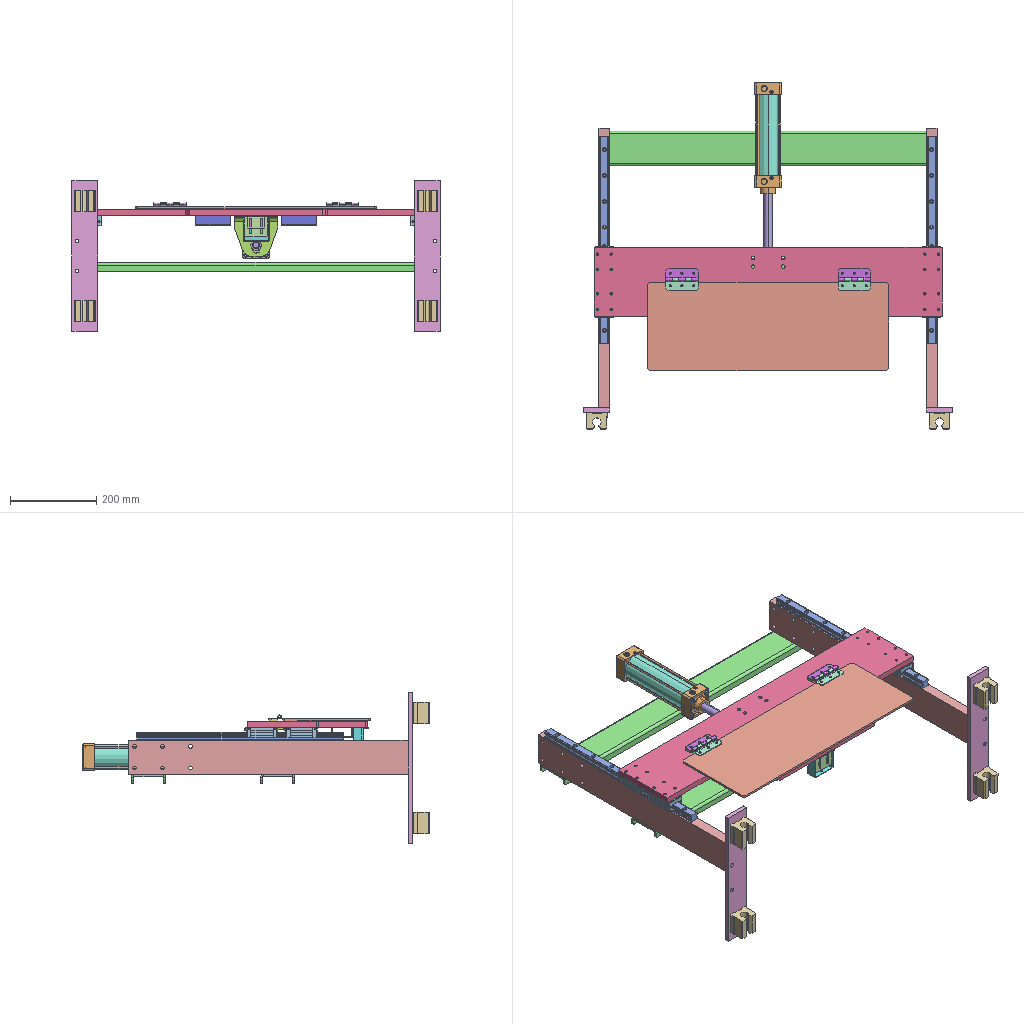Assembly | SolidWorks | 24 different items | 39 placed | box 855 x 804 x 350 mm
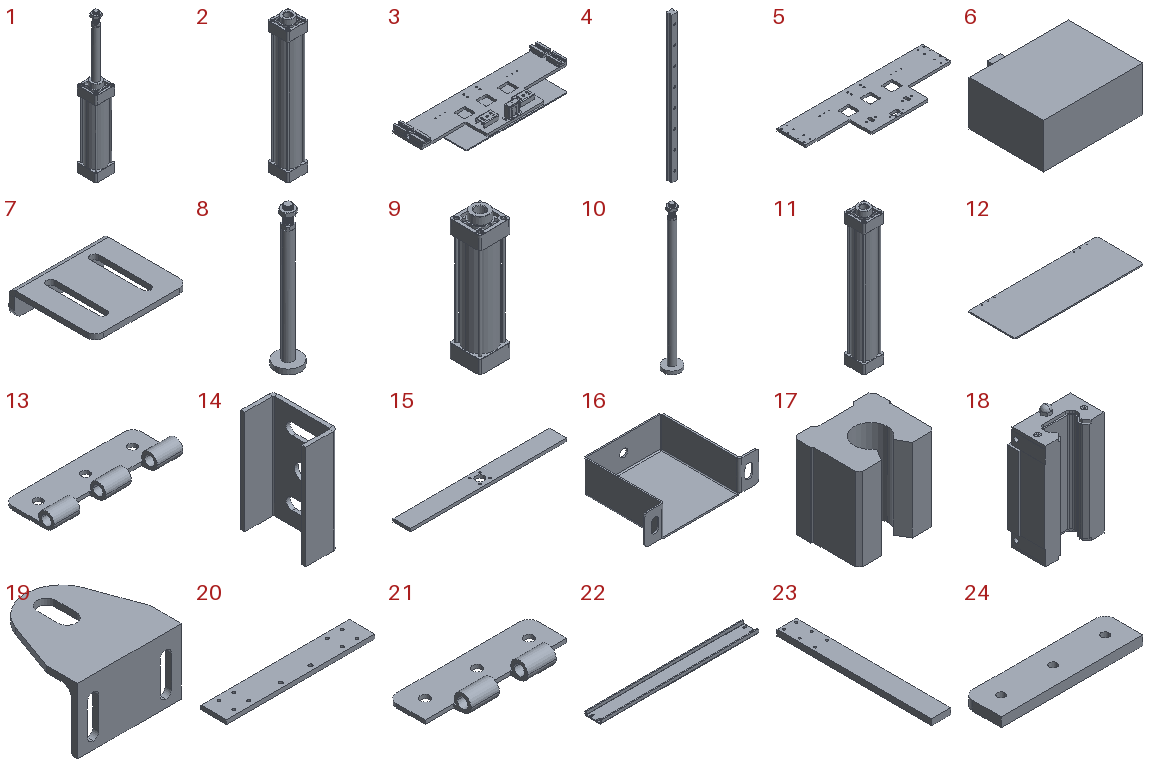Parts list (item | name | quantity | parent item | size | volume | features):
1 | (subassembly) | x1 | - | 62 x 62 x 450 mm | 443231 mm3 | -
2 | (subassembly) | x1 | - | 62 x 62 x 408 mm | 454706 mm3 | -
3 | (subassembly) | x1 | - | 808 x 294.081 x 89.45 mm | 3072025 mm3 | features ReferencePattern 5, CompositeCurve 2, LocalLPattern 1, MirrorCompFeat 1
4 | - | x2 | - | 20.703 x 18 x 480 mm | 151850 mm3 | features Chamfer 1, Extrusion 1, HoleWzd 1, LPattern 1
5 | - | x1 | in 3 | 808 x 280 x 14 mm | 2155806 mm3 | features HoleWzd 5, ICE 4, 3DProfileFeature 3, Chamfer 2, LPattern 2, Extrusion 1, Fillet 1
6 | - | x1 | in 3 | 40 x 40 x 18 mm | 21975 mm3 | features Extrusion 1, ICE 1
7 | - | x1 | in 3 | 54 x 50 x 15 mm | 8636 mm3 | features EdgeFlange 1, Extrusion 1, Fillet 1, FlatPattern 1, ICE 1, SheetMetal 1, SolidToSheetMetal 1
8 | - | x1 | in 1 | 50 x 50 x 272.5 mm | 99856 mm3 | features ICE 5, Revolution 3, RevCut 2, Chamfer 1, Helix 1, LPattern 1, MirrorPattern 1, SweepCut 1
9 | - | x1 | in 1 | 62 x 62 x 258 mm | 343374 mm3 | features ICE 11, Fillet 4, Revolution 4, MirrorPattern 3, Chamfer 2, CirPattern 2, Helix 1, RevCut 1, SweepCut 1
10 | - | x1 | - | 50 x 50 x 422.5 mm | 146980 mm3 | features ICE 5, Revolution 3, RevCut 2, Chamfer 1, Helix 1, LPattern 1, MirrorPattern 1, SweepCut 1
11 | - | x1 | - | 62 x 62 x 408 mm | 454706 mm3 | features ICE 11, Fillet 4, Revolution 4, MirrorPattern 3, Chamfer 2, CirPattern 2, Helix 1, RevCut 1, SweepCut 1
12 | - | x1 | in 3 | 560 x 205 x 5 mm | 573373 mm3 | features Extrusion 1
13 | - | x2 | in 3 | 75 x 29.3 x 9.25 mm | 4864 mm3 | features Extrusion 1, Fillet 1, ICE 1, LPattern 1
14 | - | x2 | in 3 | 25 x 50 x 80 mm | 20596 mm3 | features EdgeFlange 1, FlatPattern 1, SMBaseFlange 1, SheetMetal 1
15 | - | x1 | - | 735 x 80 x 14 mm | 799824 mm3 | features 3DProfileFeature 2, HoleWzd 2, Extrusion 1, ICE 1
16 | - | x2 | in 3 | 87.6 x 61.2 x 25 mm | 9770 mm3 | features EdgeFlange 2, Fillet 1, FlatPattern 1, ICE 1, SMBaseFlange 1, SheetMetal 1
17 | - | x4 | - | 48 x 39 x 50 mm | 66905 mm3 | features Chamfer 1, Extrusion 1, ICE 1
18 | - | x4 | in 3 | 44 x 25 x 77.9 mm | 57159 mm3 | features ICE 10, MirrorPattern 3, Chamfer 1, Extrusion 1, HoleWzd 1, Revolution 1
19 | - | x1 | - | 100 x 100 x 63 mm | 75285 mm3 | features ICE 2, 3DProfileFeature 1, WeldMemberFeat 1, WeldmentFeature 1
20 | - | x2 | - | 350 x 60 x 10 mm | 206210 mm3 | features Extrusion 1, HoleWzd 1
21 | - | x2 | in 3 | 75 x 29.3 x 9.25 mm | 4196 mm3 | features Extrusion 1, Fillet 1, ICE 1, LPattern 1
22 | - | x2 | - | 785 x 80 x 20 mm | 417138 mm3 | features EdgeFlange 1, Fillet 1, FlatPattern 1, ICE 1, SMBaseFlange 1, SheetMetal 1
23 | - | x2 | - | 80 x 650 x 25 mm | 1287489 mm3 | features HoleWzd 2, 3DProfileFeature 1, Extrusion 1, LPattern 1
24 | - | x2 | in 3 | 75 x 20 x 5 mm | 7258 mm3 | features Extrusion 1, Fillet 1
Mates (type | each side: item.copy, entity, surface, feature):
In the top assembly
Coincident | 23.1 face plane Boss-Extrude1 | 4.1 face plane Boss-Extrude1
DistanceDim | 23.1 face plane Boss-Extrude1 | 4.1 face plane Boss-Extrude1 | 2 times
Coincident | 23.2 face plane Boss-Extrude1 | 4.2 face plane Boss-Extrude1
DistanceDim | 23.2 face plane Boss-Extrude1 | 4.2 face plane Boss-Extrude1 | 2 times
Coincident | 23.1 face plane Boss-Extrude1 | 20.1 face plane Boss-Extrude1 | 2 times
Coincident | 23.2 face plane Boss-Extrude1 | 20.2 face plane Boss-Extrude1 | 2 times
Coincident | 20.1 face plane Boss-Extrude1 | 20.2 face plane Boss-Extrude1
Coincident | 23.1 face plane Boss-Extrude1 | 15.1 face plane Boss-Extrude1 | 2 times
Coincident | 23.2 face plane Boss-Extrude1 | 15.1 face plane Boss-Extrude1 | 2 times
Concentric | assembly face | 10.1 face | 2 times
LimitDistanceDim | assembly face | 10.1 face
DistanceDim | 20.2 face plane Boss-Extrude1 | 23.2 face plane Boss-Extrude1
Coincident | 15.1 face plane Boss-Extrude1 | 9.1 face plane Boss-Extrude1
Concentric | 15.1 face cylinder Cut-Extrude1 | 9.1 edge
Concentric | 23.1 edge | 15.1 face cylinder M8 Tapped Hole1
Concentric | 23.2 face cylinder Ø9.0 (9) Diameter Hole1 | 15.1 face cylinder M8 Tapped Hole2
Coincident | 23.2 face plane Boss-Extrude1 | 22.1 face plane Base-Flange1
Width | 23.2 face plane Boss-Extrude1 | 23.1 face plane Boss-Extrude1 | 22.1 face plane Base-Flange1 | 22.1 face plane Base-Flange1
Coincident | 4.1 face plane Boss-Extrude1 | 18.1 face plane Cut-Extrude2
Width | 18.1 face plane Cut-Extrude6 | 18.1 face plane Cut-Extrude6 | 4.1 face plane Boss-Extrude1 | 4.1 face plane Boss-Extrude1
Concentric | 20.1 face cylinder Boss-Extrude1 | 17.1 face cylinder Cut-Extrude1 | 2 times
Coincident | 19.1 face plane Hot-rolled unequal angle gb∕t706-2008 100 X 63 X 6(1) | 5.1 face plane Boss-Extrude1
Slot | 19.1 face cylinder Cut-Extrude2 | 5.1 face cylinder M10 Tapped Hole2
Slot | 5.1 face cylinder M10 Tapped Hole2 | 19.1 face cylinder Cut-Extrude2
Concentric | 15.1 face cylinder Cut-Extrude1 | 8.1 face cylinder Revolve1
Coincident | 20.1 face plane Boss-Extrude1 | 17.1 face plane Boss-Extrude1
DistanceDim | 19.1 face plane Hot-rolled unequal angle gb∕t706-2008 100 X 63 X 6(1) | 15.1 face plane Boss-Extrude1
Slot | 22.1 face cylinder Cut-Extrude1 | 23.2 face cylinder M8 Tapped Hole1
Slot | 22.2 face cylinder Cut-Extrude1 | 23.2 face cylinder LPattern1
Coincident | 23.2 face plane Boss-Extrude1 | 22.2 face plane Base-Flange1
Slot | 23.2 face cylinder LPattern1 | 22.2 face cylinder Cut-Extrude1
In subassembly 1
Concentric | 9.2 face cylinder Revolve2 | 8.2 face cylinder Revolve1
LimitDistanceDim | 9.2 face plane Boss-Extrude2 | 8.2 face plane Revolve1
In subassembly 3
Concentric | 5.2 face cylinder LPattern3 | 18.2 face cylinder threaded hole 1 | 2 times
Coincident | 5.2 face plane Boss-Extrude1 | 18.2 face plane Boss-Extrude1
Concentric | 5.2 edge | 18.3 face cylinder threaded hole 1 | 2 times
Coincident | 5.2 face plane Boss-Extrude1 | 18.3 face plane Boss-Extrude1
Coincident | 5.2 face plane Boss-Extrude1 | 24.1 face plane Boss-Extrude1
Concentric | 5.2 face cylinder M5 Tapped Hole1 | 24.1 face cylinder Boss-Extrude1 | 2 times
Coincident | 5.2 face plane Boss-Extrude1 | 24.2 face plane Boss-Extrude1
Concentric | 5.2 face cylinder M5 Tapped Hole1 | 24.2 face cylinder Boss-Extrude1 | 2 times
Coincident | 24.1 face plane Boss-Extrude1 | 13.1 face plane Boss-Extrude1
Concentric | 24.1 face cylinder Boss-Extrude1 | 13.1 face cylinder Boss-Extrude1 | 2 times
Concentric | 13.1 face cylinder LPattern1 | 21.1 face cylinder LPattern1
Coincident | 13.1 face plane Boss-Extrude2 | 21.1 face plane LPattern1
Concentric | 21.1 face cylinder Boss-Extrude1 | 12.1 face cylinder Boss-Extrude1
Coincident | 21.1 face plane Boss-Extrude1 | 12.1 face plane Boss-Extrude1
Concentric | 21.2 face cylinder Boss-Extrude1 | 12.1 face cylinder Boss-Extrude1
Concentric | 5.2 face cylinder Cut-Extrude1 | 7.1 face cylinder Cut-Extrude1 | 2 times
Coincident | 5.2 face plane Boss-Extrude1 | 7.1 face plane Edge-Flange2
Coincident | 7.1 face plane Convert Entities1 | 6.1 face plane Boss-Extrude1
Coincident | 5.2 face plane Boss-Extrude1 | 6.1 face plane Boss-Extrude1
Width | 6.1 face plane Boss-Extrude1 | 6.1 face plane Boss-Extrude1 | 7.1 face plane Convert Entities1 | 7.1 face plane Convert Entities1
Coincident | 5.2 face plane Boss-Extrude1 | 16.1 face plane Edge-Flange2
Coincident | 5.2 face plane Boss-Extrude1 | 14.1 face plane Edge-Flange1
Slot | 14.1 face cylinder Base-Flange1 | 5.2 face cylinder Cut-Extrude1
Parallel | 5.2 face plane Boss-Extrude2 | 14.2 face plane Edge-Flange1